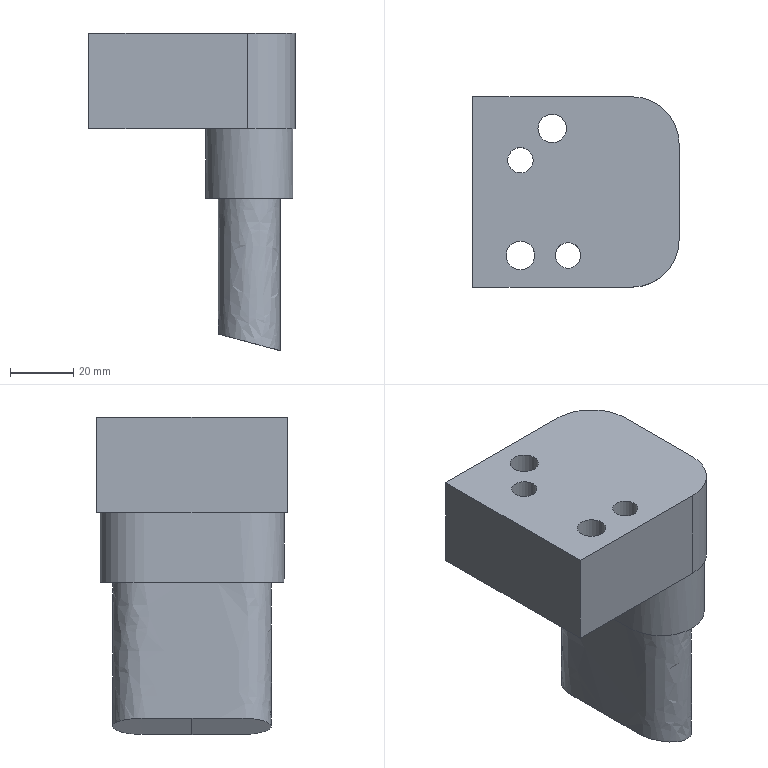Part | NX | features solid 2 | 1 solid | 25 faces | box 65 x 60 x 99.929 mm | volume 175348 mm3 | plane 9 | cylinder 8 | spline 8 | commonest cylinder face diameters 8 x2 9 x2 14 x2 30 x2